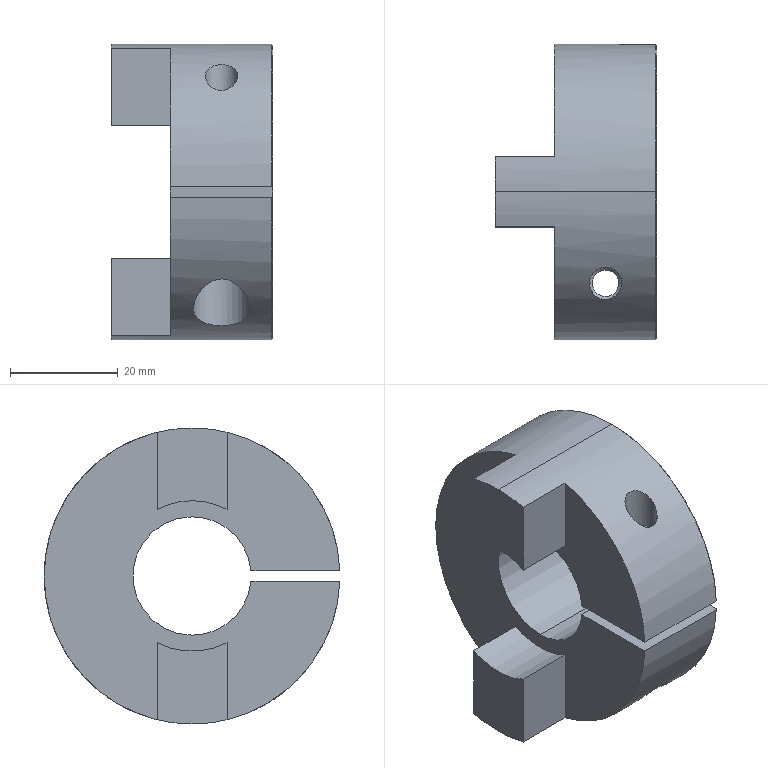Part | STEP file | 0229_Z_MFJC55-20-22_4 | 1 solid | 35 faces | box 30 x 54.982 x 55 mm | volume 39507 mm3 | cylinder 17 | plane 11 | cone 7 | commonest cylinder face diameters 6 x4 22 x3 28 x3 55 x3 4.917 x2 10.5 x2